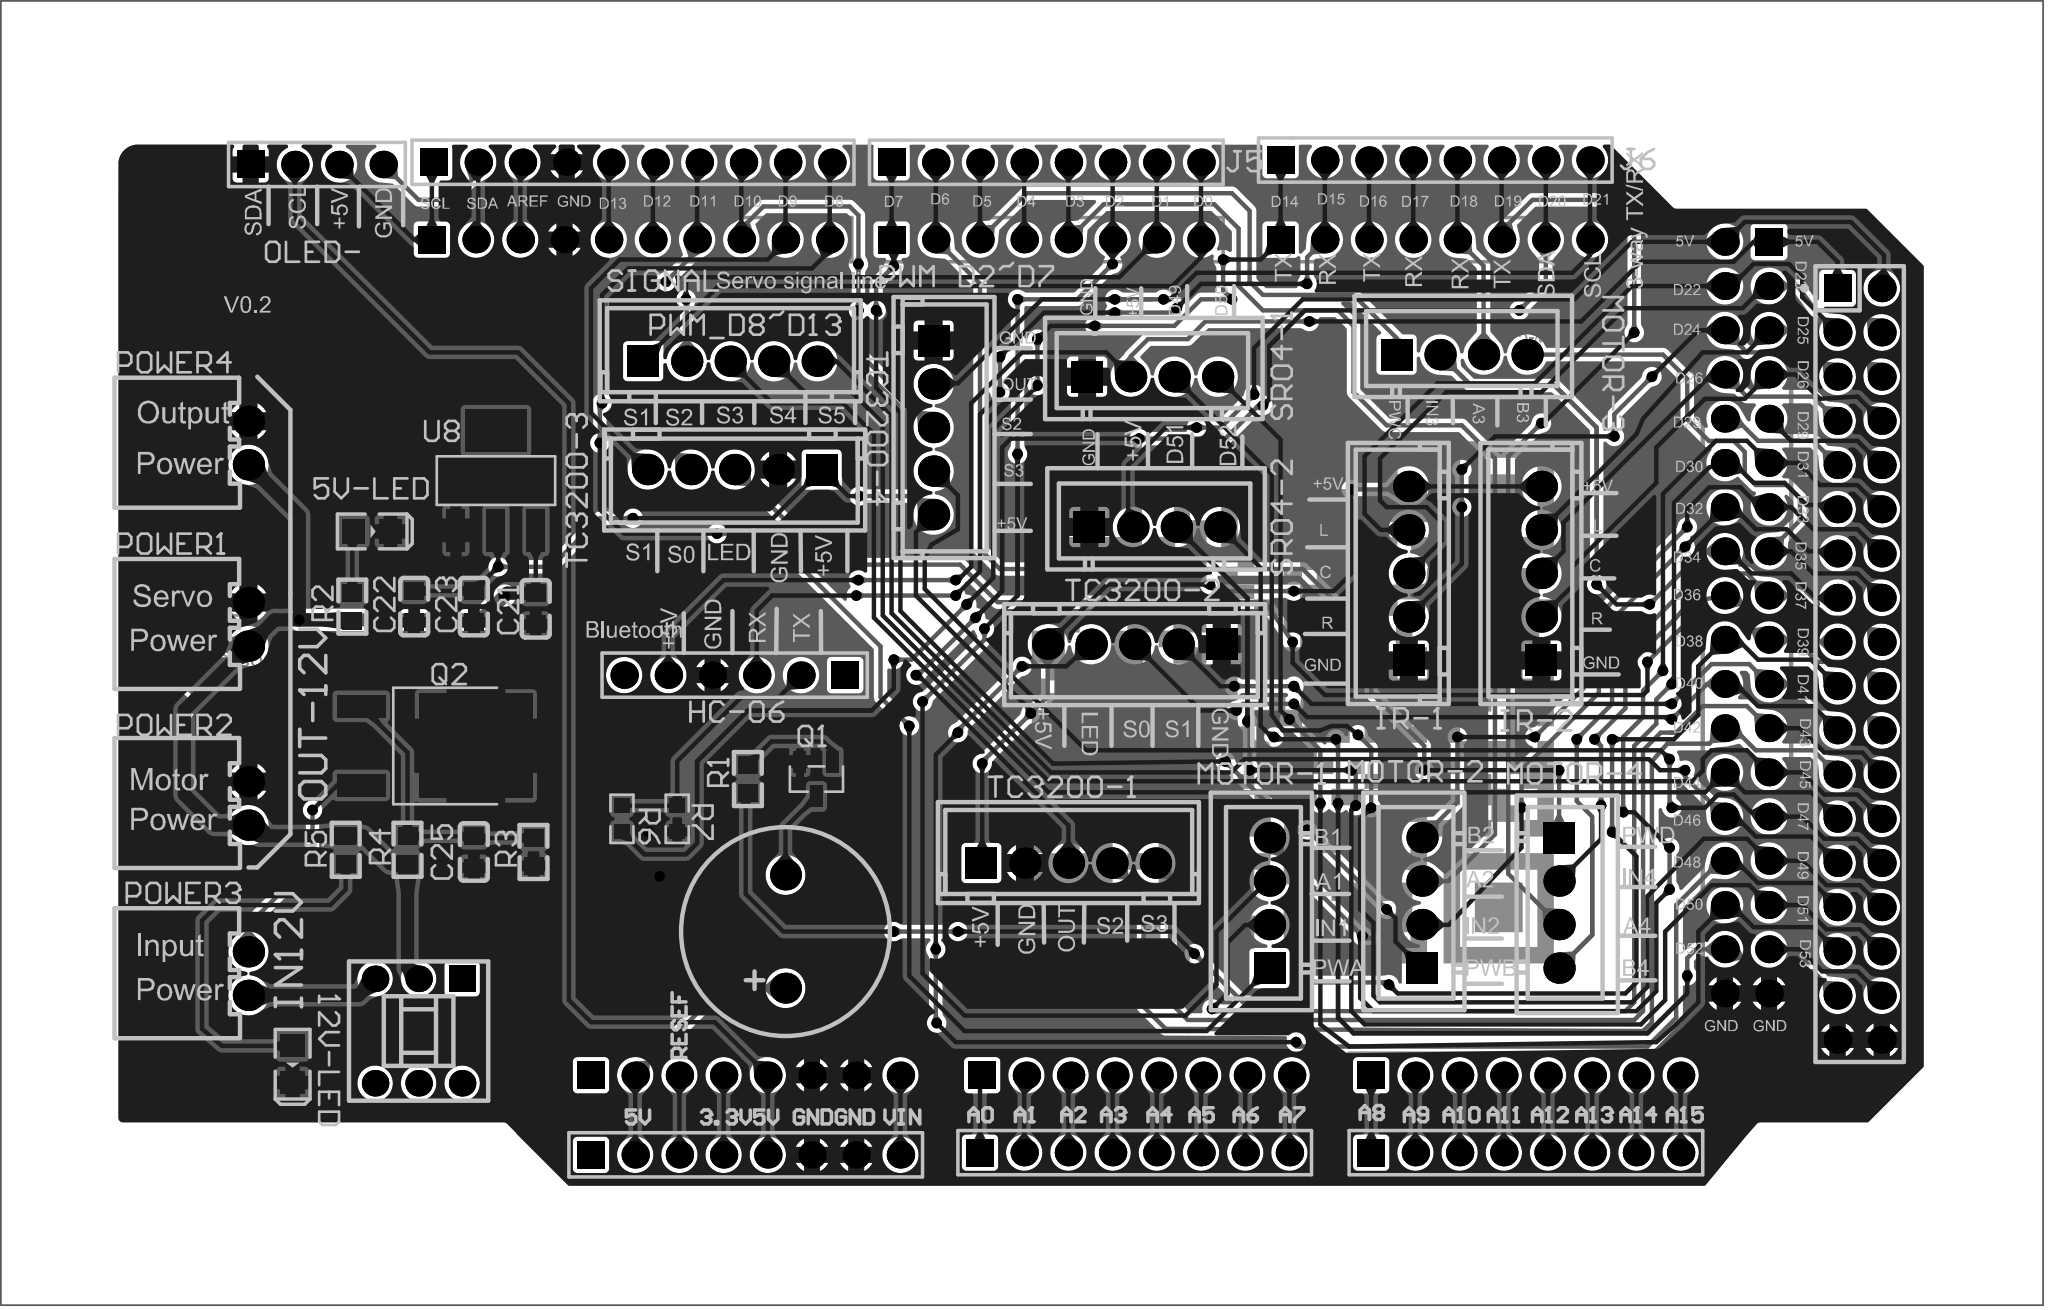Circuit board layout | Altium Designer
Layer stack:
# Altium Designer layer stack of  (unit mm; dielectric type: 0 none, 1 core, 2 prepreg, 3 surface material)
index,name,kind,layer,copper_thickness_mm,dielectric_type,dielectric_thickness_mm,dielectric_material,dielectric_constant
0,Top Silkscreen Layer,other,,,,,,
1,Top Paste Mask Layer,other,,,,,,
2,Top Solder Mask Layer,dielectric,,,3,0,,0
3,Top Layer,copper,Top Layer,0,,,,
4,Substrate-1,dielectric,,,3,0,,0
5,Bottom Layer,copper,Bottom Layer,0,,,,
6,Bottom Solder Mask Layer,dielectric,,,3,0,,0
7,Bottom Paste Mask Layer,other,,,,,,
8,Bottom Silkscreen Layer,other,,,,,,
# drill layer pairs: low layer,high layer
drill_pair,Top Layer,Bottom Layer
Part placement:
Designator,Comment,Layer,Footprint,Center-X(mm),Center-Y(mm),Rotation
POWER4,XH-2AW,TopLayer,CONN-TH_2P-P2.50_XH-2AW,84.074,119.38,90
+12,Pad,BottomLayer,焊盘,79.502,109.601,180
5V-LED,LED-0805_R,TopLayer,LED0805_RED,91.186,114.3,0
12V-LED,LED-0805_R,TopLayer,LED0805_RED,86.614,83.693,270
R2,200,TopLayer,R0603,90.043,109.982,270
R5,4.7k,TopLayer,R0603,89.662,96.012,270
OLED-,OLED_,TopLayer,HDR-F-2.54_1X4,88.011,135.382,0
POWER1,XH-2AW,TopLayer,CONN-TH_2P-P2.50_XH-2AW,84.074,108.966,90
POWER2,XH-2AW,TopLayer,CONN-TH_2P-P2.50_XH-2AW,84.074,98.679,90
POWER3,XH-2AW,TopLayer,CONN-TH_2P-P2.50_XH-2AW,84.074,88.9,90
H2,X6521WV-2×18H-C30D60,TopLayer,HDR-TH_36P-2.54-V-M-R2-C18-S2.54,176.657,106.68,270
BUZZER1,GMC1205YA-16R2048,TopLayer,BUZ-TH_BD12.0-P6.50-D0.6-FD,114.935,91.313,90
C21,100nf,TopLayer,C0603,100.584,109.855,90
C22,100nf,TopLayer,C0603,93.599,109.982,90
C23,100nf,TopLayer,C0603,97.028,109.982,90
C25,100nf,TopLayer,C0603,97.028,95.885,90
HC-06,Bluetooth,TopLayer,HDR-F-2.54_1X6,112.014,106.045,180
IR-1,XH-5A_C722874,TopLayer,CONN-TH_XH-5A,150.749,111.887,90
IR-2,XH-5A_C722874,TopLayer,CONN-TH_XH-5A,158.369,111.887,90
SIGNAL,XH-5A_C722874,TopLayer,CONN-TH_XH-5A,111.76,124.079,0
TC3200-1,XH-5A_C722874,TopLayer,CONN-TH_XH-5A,131.191,95.25,0
TC3200-2,XH-5A_C722874,TopLayer,CONN-TH_XH-5A,135.001,107.823,180
TC3200-3,XH-5A_C722874,TopLayer,CONN-TH_XH-5A,112.014,117.856,180
TC3200-4,XH-5A_C722874,TopLayer,CONN-TH_XH-5A,123.444,120.269,270
J5,PWM D2~D7,TopLayer,HDR-M-2.54_1X8,129.921,135.509,0
J6,3-way TX/RX,TopLayer,HDR-M-2.54_1X8,152.273,135.636,0
J7,HDR-M-2.54_1x8,TopLayer,HDR-M-2.54_1X8,157.48,78.613,0
J12,HDR-M-2.54_1x8,TopLayer,HDR-M-2.54_1X8,112.649,78.486,0
J13,HDR-M-2.54_1x8,TopLayer,HDR-M-2.54_1X8,135.001,78.613,0
J3,PWM_D8~D13,TopLayer,HDR-M-2.54_1X10,106.172,135.509,0
MOTOR-1,MOTOR-1,TopLayer,CONN-TH_4P-P2.50_XH-4A,142.748,92.964,90
MOTOR-2,MOTOR-2,TopLayer,CONN-TH_4P-P2.50_XH-4A,151.511,92.964,90
MOTOR-3,MOTOR-3,TopLayer,CONN-TH_4P-P2.50_XH-4A,153.797,124.46,0
MOTOR-4,MOTOR-4,TopLayer,CONN-TH_4P-P2.50_XH-4A,159.385,92.964,270
SRO4-1,Ultrasonic module,TopLayer,CONN-TH_4P-P2.50_XH-4A,136.017,123.19,0
SRO4-2,Ultrasonic module,TopLayer,CONN-TH_4P-P2.50_XH-4A,136.144,114.554,0
Q1,S8050,TopLayer,SOT-23-3_L2.9-W1.3-P1.90-LS2.4-BR,116.713,100.076,90
Q2,KIA50N03A,TopLayer,TO-252-2_L6.6-W6.1-P4.57-LS9.9-TL-CW,93.853,101.981,0
R1,10k,TopLayer,R0603,112.776,100.076,90
R3,10K,TopLayer,R0603,100.457,95.885,90
R4,10k,TopLayer,R0603,93.218,96.012,90
R6,10K,TopLayer,R0603,105.537,97.79,270
R7,20K,TopLayer,R0603,108.712,97.79,90
SW1,XKB8080-Z,TopLayer,SW-TH_6P-L8.0-W8.0-P2.50,93.853,85.598,180
U8,AMS1117-5.0,TopLayer,SOT-223_L6.5-W3.5-P2.30-LS7.0-BR,98.298,117.221,270
-GND,Pad,BottomLayer,焊盘,79.502,104.267,180
J8,HDR-M-2.54_1x8,BottomLayer,HDR-M-2.54_1X8,135.128,83.058,0
H1,X6521WV-2×18H-C30D60,BottomLayer,HDR-TH_36P-2.54-V-M-R2-C18-S2.54,170.18,109.347,270
J1,3-way TX/RX,BottomLayer,HDR-M-2.54_1X8,152.273,131.064,0
J2,PWM D2~D7,BottomLayer,HDR-M-2.54_1X8,129.921,131.064,0
J9,HDR-M-2.54_1x8,BottomLayer,HDR-M-2.54_1X8,112.649,83.058,0
J14,HDR-M-2.54_1x8,BottomLayer,HDR-M-2.54_1X8,157.48,83.058,0
J4,PWM_D8~D13,BottomLayer,HDR-M-2.54_1X10,106.045,131.064,0
Pad and via stacks:
# Altium Designer via and pad stacks of  (unit mm). Each distinct definition once, with the count of objects using it.
# via: kind,start_layer,end_layer,hole_mm,diameter_mm,mode(0 simple;1 top-mid-bottom;2 full stack),diameter_per_layer,count,example_net
# pad: kind,layer,hole_mm,hole_type(0 round;1 square;2 slot),plating,top_size,top_shape(1 round;2 rect;3 octagon;9 rounded rect),mid_size,bottom_size,mode,footprint,size_per_layer,count,example
pad,Multi-Layer,1.199,0,plated,1.8x1.8,1,1.8x1.8,1.8x1.8,0,CONN-TH_2P-P2.50_XH-2AW,,8,POWER4.1
pad,Multi-Layer,0.889,0,plated,1.575x1.575,2,1.575x1.575,1.575x1.575,0,HDR-F-2.54_1X4,,1,OLED-.1
pad,Multi-Layer,0.889,0,plated,1.575x1.575,1,1.575x1.575,1.575x1.575,0,HDR-F-2.54_1X4,,3,OLED-.2
pad,Multi-Layer,1.05,0,plated,1.6x1.6,2,1.6x1.6,1.6x1.6,0,HDR-TH_36P-2.54-V-M-R2-C18-S2.54,,2,H2.1
pad,Multi-Layer,1.05,0,plated,1.6x1.6,1,1.6x1.6,1.6x1.6,0,HDR-TH_36P-2.54-V-M-R2-C18-S2.54,,70,H2.2
pad,Multi-Layer,0.8992,0,plated,1.778x1.778,1,1.778x1.778,1.778x1.778,0,BUZ-TH_BD12.0-P6.50-D0.6-FD,,2,BUZZER1.1
pad,Multi-Layer,0.889,0,plated,1.575x1.575,1,1.575x1.575,1.575x1.575,0,HDR-F-2.54_1X6,,5,HC-06.6
pad,Multi-Layer,0.889,0,plated,1.575x1.575,2,1.575x1.575,1.575x1.575,0,HDR-F-2.54_1X6,,1,HC-06.1
pad,Multi-Layer,1.2,0,plated,1.8x1.8,1,1.8x1.8,1.8x1.8,0,CONN-TH_XH-5A,,28,IR-1.3
pad,Multi-Layer,1.2,0,plated,1.8x1.8,2,1.8x1.8,1.8x1.8,0,CONN-TH_XH-5A,,7,IR-1.1
pad,Multi-Layer,0.889,0,plated,1.575x1.575,2,1.575x1.575,1.575x1.575,0,HDR-M-2.54_1X8,,10,J5.1
pad,Multi-Layer,0.889,0,plated,1.575x1.575,1,1.575x1.575,1.575x1.575,0,HDR-M-2.54_1X8,,70,J5.2
pad,Multi-Layer,0.889,0,plated,1.575x1.575,1,1.575x1.575,1.575x1.575,0,HDR-M-2.54_1X10,,18,J3.10
pad,Multi-Layer,0.9449,0,plated,1.575x1.575,2,1.575x1.575,1.575x1.575,0,HDR-M-2.54_1X10,,1,J3.1
pad,Multi-Layer,1.199,0,plated,1.8x1.8,2,1.8x1.8,1.8x1.8,0,CONN-TH_4P-P2.50_XH-4A,,6,MOTOR-1.1
pad,Multi-Layer,1.199,0,plated,1.8x1.8,1,1.8x1.8,1.8x1.8,0,CONN-TH_4P-P2.50_XH-4A,,18,MOTOR-1.2
pad,Multi-Layer,1,0,plated,1.524x1.524,1,1.524x1.524,1.524x1.524,0,SW-TH_6P-L8.0-W8.0-P2.50,,5,SW1.3
pad,Multi-Layer,1,0,plated,1.524x1.524,2,1.524x1.524,1.524x1.524,0,SW-TH_6P-L8.0-W8.0-P2.50,,1,SW1.1
pad,Multi-Layer,0.889,0,plated,1.575x1.575,2,1.575x1.575,1.575x1.575,0,HDR-M-2.54_1X10,,1,J4.1
pad,Bottom Layer,0,0,plated,2.54x1.524,1,2.54x1.524,2.54x1.524,0,\u00BA\u00B8\u00C5\u00CC,,2,+12.1
pad,Top Layer,0,0,plated,1.3x1.399,2,1.3x1.399,1.3x1.399,0,LED0805_RED,,4,5V-LED.1
pad,Top Layer,0,0,plated,1x1.1,2,1x1.1,1x1.1,0,R0603,,10,R2.2
pad,Top Layer,0,0,plated,1x1.1,2,1x1.1,1x1.1,0,C0603,,8,C21.1
pad,Top Layer,0,0,plated,1.25x0.7,2,1.25x0.7,1.25x0.7,0,SOT-23-3_L2.9-W1.3-P1.90-LS2.4-BR,,3,Q1.1
pad,Top Layer,0,0,plated,6.5x6,2,6.5x6,6.5x6,0,TO-252-2_L6.6-W6.1-P4.57-LS9.9-TL-CW,,1,Q2.2
pad,Top Layer,0,0,plated,2.8x1.3,2,2.8x1.3,2.8x1.3,0,TO-252-2_L6.6-W6.1-P4.57-LS9.9-TL-CW,,2,Q2.1
pad,Top Layer,0,0,plated,0.8065x0.864,2,0.8065x0.864,0.8065x0.864,0,R0603,,4,R6.2
pad,Top Layer,0,0,plated,2.465x1.05,2,2.465x1.05,2.465x1.05,0,SOT-223_L6.5-W3.5-P2.30-LS7.0-BR,,3,U8.1
pad,Top Layer,0,0,plated,2.465x3.54,2,2.465x3.54,2.465x3.54,0,SOT-223_L6.5-W3.5-P2.30-LS7.0-BR,,1,U8.4
via,Top Layer,Bottom Layer,0.3048,0.6096,0,,118,OUT1_+5V
Copper pours:
name,layer,net,type(0 solid;1 hatched;2 none)
Bottom Layer-GND,Bottom Layer,GND,0
Top Layer-GND,Top Layer,GND,0
Design rules, without the lines most boards share:
# Altium Designer design rules of  (exported by Altium Designer, unit mm)
# columns: name | kind | enabled | priority | scope1 | scope2 | descriptor | typed fields (field=value)
DiffPairsRouting | 51 | enabled | 1 | All | All | Differential Pairs Uncoupled Length using the Gap Constraints (Min=10mil) (Max=10mil) (Prefered=10mil)  and Width Constraints (Min=15mil) (Max=15mil) (Prefered=15mil) (All) |
SolderMaskExpansion | 13 | enabled | 1 | All | All | Solder Mask Expansion (Expansion =4mil) (All) | expansion=0.1016
PasteMaskExpansion | 14 | enabled | 1 | All | All | Paste Mask Expansion (Expansion =0mil) (All) | expansion=0
RoutingVias | 11 | enabled | 1 | All | All | Routing Via (MinHoleWidth=28mil) (MaxHoleWidth=28mil) (PreferredHoleWidth=28mil) (MinWidth=50mil) (MaxWidth=50mil) (PreferedWidth=50mil) (All) | via_min_hole=0.7112 via_max_hole=0.7112 via_preferred_diameter=1.27 via_preferred_hole=0.7112
Width | 2 | enabled | 1 | All | All | Width Constraint (Min=10mil) (Max=10mil) (Preferred=10mil) (All) |
PolygonConnect | 20 | enabled | 1 | All | All | Polygon Connect Rule(Relief Connect )(Conductor Width=10mil) (Relief Angle=90 Angle) (Entries=4) (Air Gap Width=10mil) (All),(All) | connect_style(0=relief,1=direct,2=none)=0 relief_conductor_width=0.254 relief_entries=4
PlaneConnect | 6 | enabled | 1 | All | All | Power Plane Connect Rule(Relief Connect )(Expansion=20mil) (Conductor Width=10mil) (Air Gap=10mil) (Entries=4) (All) | relief_conductor_width=0.254 relief_entries=4 relief_expansion=0.508
Clearance | 0 | enabled | 1 | All | All | Clearance Constraint (Gap=10mil) (All),(All) | gap=0.254
Default | 52 | disabled | 1 | All | All | Hole To Hole Clearance (Gap=0mil) (Disabled)(All),(All) | gap=0
gge14896 | 52 | disabled | 2 | All | All | Hole To Hole Clearance (Gap=0mil) (Disabled)(All),(All) | gap=0
gge14902 | 52 | disabled | 3 | All | All | Hole To Hole Clearance (Gap=0mil) (Disabled)(All),(All) | gap=0
Common | 52 | enabled | 4 | All | All | Hole To Hole Clearance (Gap=11.8mil) (All),(All) | gap=0.2997